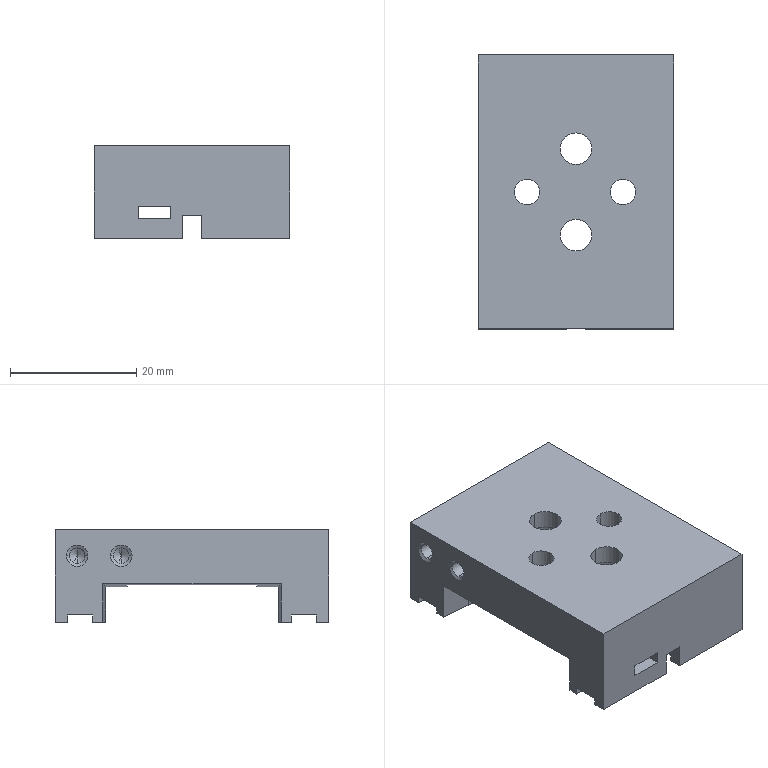Part | NX | 1 solid | 146 faces | box 31 x 43.4 x 14.65 mm | volume 12601 mm3 | plane 57 | cylinder 55 | cone 34 | commonest cylinder face diameters 2.5 x43 4 x4 5 x4 9 x4